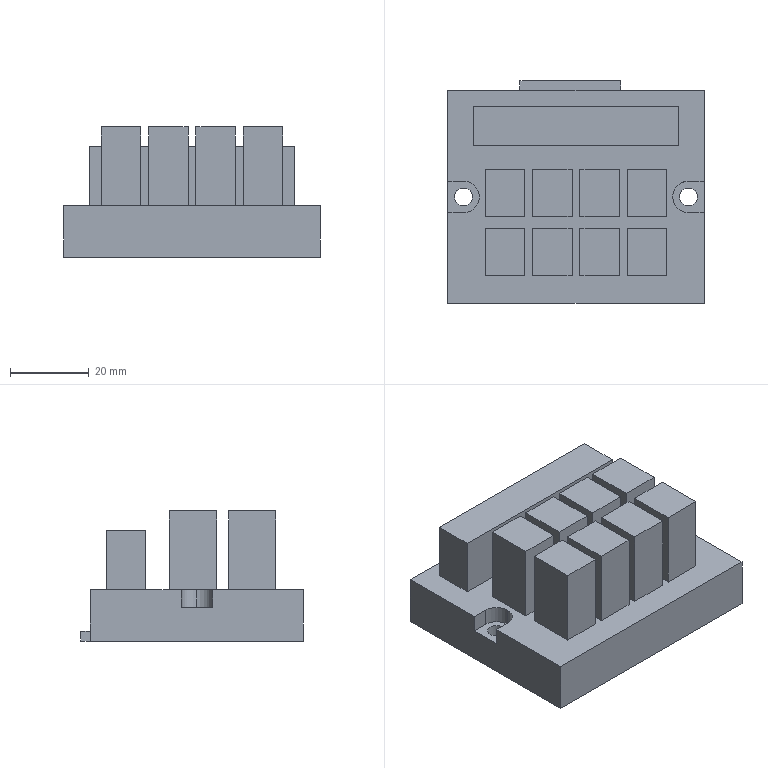Part | STEP file | 11-T08011 | 1 solid | 68 faces | box 65 x 56.5 x 33 mm | volume 72013 mm3 | plane 61 | cylinder 7 | commonest cylinder face diameters 4.5 x4 8 x3